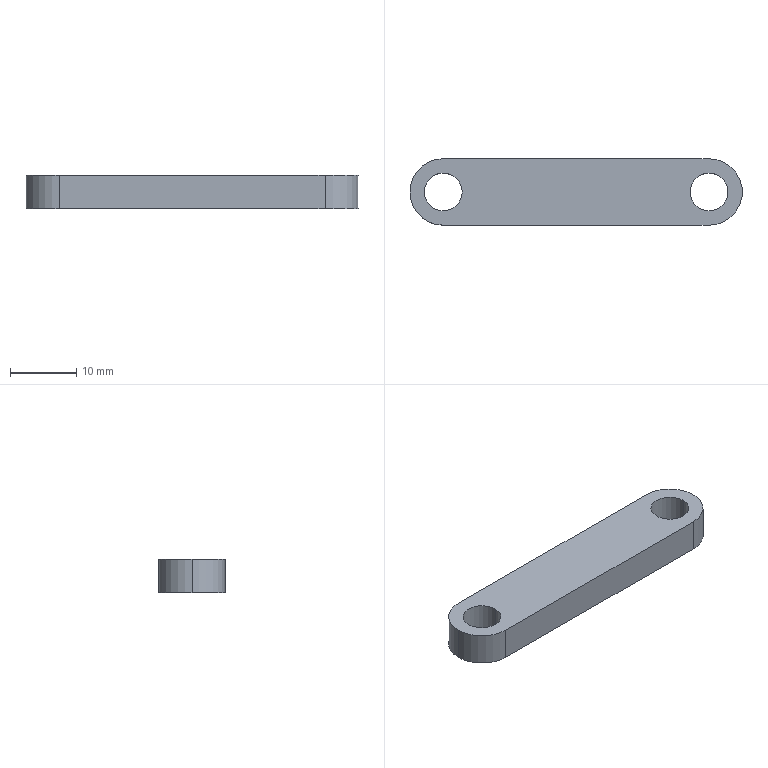Part | SolidWorks | features BaseBody 1 | 1 solid | 11 faces | box 50 x 10 x 5 mm | volume 2138 mm3 | cylinder 7 | plane 4 | commonest cylinder face diameters 5.7 x4 10 x3
STEP:
#1=CARTESIAN_POINT('',(17.15,0.,2.5));
#2=VERTEX_POINT('',#1);
#3=CARTESIAN_POINT('',(22.85,0.,2.5));
#4=VERTEX_POINT('',#3);
#5=CARTESIAN_POINT('',(20.,0.,2.5));
#6=DIRECTION('',(0.,0.,1.));
#7=DIRECTION('',(1.,0.,0.));
#8=AXIS2_PLACEMENT_3D('',#5,#6,#7);
#9=CIRCLE('',#8,2.85);
#10=EDGE_CURVE('',#2,#4,#9,.T.);
#11=ORIENTED_EDGE('',*,*,#10,.T.);
#12=CARTESIAN_POINT('',(22.85,0.,-2.5));
#13=VERTEX_POINT('',#12);
#14=CARTESIAN_POINT('',(22.85,0.,2.5));
#15=DIRECTION('',(0.,0.,-1.));
#16=VECTOR('',#15,1000.);
#17=LINE('',#14,#16);
#18=EDGE_CURVE('',#4,#13,#17,.T.);
#19=ORIENTED_EDGE('',*,*,#18,.T.);
#20=CARTESIAN_POINT('',(17.15,0.,-2.5));
#21=VERTEX_POINT('',#20);
#22=CARTESIAN_POINT('',(20.,0.,-2.5));
#23=DIRECTION('',(0.,0.,1.));
#24=DIRECTION('',(1.,0.,0.));
#25=AXIS2_PLACEMENT_3D('',#22,#23,#24);
#26=CIRCLE('',#25,2.85);
#27=EDGE_CURVE('',#21,#13,#26,.T.);
#28=ORIENTED_EDGE('',*,*,#27,.F.);
#29=CARTESIAN_POINT('',(17.15,0.,2.5));
#30=DIRECTION('',(0.,0.,-1.));
#31=VECTOR('',#30,1000.);
#32=LINE('',#29,#31);
#33=EDGE_CURVE('',#2,#21,#32,.T.);
#34=ORIENTED_EDGE('',*,*,#33,.F.);
#35=EDGE_LOOP('',(#11,#19,#28,#34));
#36=FACE_OUTER_BOUND('',#35,.T.);
#37=CARTESIAN_POINT('',(20.,0.,2.5));
#38=DIRECTION('',(0.,0.,-1.));
#39=DIRECTION('',(-1.,0.,0.));
#40=AXIS2_PLACEMENT_3D('',#37,#38,#39);
#41=CYLINDRICAL_SURFACE('',#40,2.85);
#42=ADVANCED_FACE('',(#36),#41,.F.);
#43=CARTESIAN_POINT('',(-22.85,0.,2.5));
#44=VERTEX_POINT('',#43);
#45=CARTESIAN_POINT('',(-17.15,0.,2.5));
#46=VERTEX_POINT('',#45);
#47=CARTESIAN_POINT('',(-20.,0.,2.5));
#48=DIRECTION('',(0.,0.,1.));
#49=DIRECTION('',(1.,0.,0.));
#50=AXIS2_PLACEMENT_3D('',#47,#48,#49);
#51=CIRCLE('',#50,2.85);
#52=EDGE_CURVE('',#44,#46,#51,.T.);
#53=ORIENTED_EDGE('',*,*,#52,.T.);
#54=CARTESIAN_POINT('',(-17.15,0.,-2.5));
#55=VERTEX_POINT('',#54);
#56=CARTESIAN_POINT('',(-17.15,0.,2.5));
#57=DIRECTION('',(0.,0.,-1.));
#58=VECTOR('',#57,1000.);
#59=LINE('',#56,#58);
#60=EDGE_CURVE('',#46,#55,#59,.T.);
#61=ORIENTED_EDGE('',*,*,#60,.T.);
#62=CARTESIAN_POINT('',(-22.85,0.,-2.5));
#63=VERTEX_POINT('',#62);
#64=CARTESIAN_POINT('',(-20.,0.,-2.5));
#65=DIRECTION('',(0.,0.,1.));
#66=DIRECTION('',(1.,0.,0.));
#67=AXIS2_PLACEMENT_3D('',#64,#65,#66);
#68=CIRCLE('',#67,2.85);
#69=EDGE_CURVE('',#63,#55,#68,.T.);
#70=ORIENTED_EDGE('',*,*,#69,.F.);
#71=CARTESIAN_POINT('',(-22.85,0.,2.5));
#72=DIRECTION('',(0.,0.,-1.));
#73=VECTOR('',#72,1000.);
#74=LINE('',#71,#73);
#75=EDGE_CURVE('',#44,#63,#74,.T.);
#76=ORIENTED_EDGE('',*,*,#75,.F.);
#77=EDGE_LOOP('',(#53,#61,#70,#76));
#78=FACE_OUTER_BOUND('',#77,.T.);
#79=CARTESIAN_POINT('',(-20.,0.,2.5));
#80=DIRECTION('',(0.,0.,-1.));
#81=DIRECTION('',(-1.,0.,0.));
#82=AXIS2_PLACEMENT_3D('',#79,#80,#81);
#83=CYLINDRICAL_SURFACE('',#82,2.85);
#84=ADVANCED_FACE('',(#78),#83,.F.);
#85=CARTESIAN_POINT('',(-25.,0.,2.5));
#86=VERTEX_POINT('',#85);
#87=CARTESIAN_POINT('',(-20.,-5.,2.5));
#88=VERTEX_POINT('',#87);
#89=CARTESIAN_POINT('',(-20.,0.,2.5));
#90=DIRECTION('',(0.,0.,1.));
#91=DIRECTION('',(1.,0.,0.));
#92=AXIS2_PLACEMENT_3D('',#89,#90,#91);
#93=CIRCLE('',#92,5.);
#94=EDGE_CURVE('',#86,#88,#93,.T.);
#95=ORIENTED_EDGE('',*,*,#94,.F.);
#96=CARTESIAN_POINT('',(-25.,0.,-2.5));
#97=VERTEX_POINT('',#96);
#98=CARTESIAN_POINT('',(-25.,0.,2.5));
#99=DIRECTION('',(0.,0.,-1.));
#100=VECTOR('',#99,1000.);
#101=LINE('',#98,#100);
#102=EDGE_CURVE('',#86,#97,#101,.T.);
#103=ORIENTED_EDGE('',*,*,#102,.T.);
#104=CARTESIAN_POINT('',(-20.,-5.,-2.5));
#105=VERTEX_POINT('',#104);
#106=CARTESIAN_POINT('',(-20.,0.,-2.5));
#107=DIRECTION('',(0.,0.,1.));
#108=DIRECTION('',(1.,0.,0.));
#109=AXIS2_PLACEMENT_3D('',#106,#107,#108);
#110=CIRCLE('',#109,5.);
#111=EDGE_CURVE('',#97,#105,#110,.T.);
#112=ORIENTED_EDGE('',*,*,#111,.T.);
#113=CARTESIAN_POINT('',(-20.,-5.,2.5));
#114=DIRECTION('',(0.,0.,-1.));
#115=VECTOR('',#114,1000.);
#116=LINE('',#113,#115);
#117=EDGE_CURVE('',#88,#105,#116,.T.);
#118=ORIENTED_EDGE('',*,*,#117,.F.);
#119=EDGE_LOOP('',(#95,#103,#112,#118));
#120=FACE_OUTER_BOUND('',#119,.T.);
#121=CARTESIAN_POINT('',(-20.,0.,2.5));
#122=DIRECTION('',(0.,0.,-1.));
#123=DIRECTION('',(-1.,0.,0.));
#124=AXIS2_PLACEMENT_3D('',#121,#122,#123);
#125=CYLINDRICAL_SURFACE('',#124,5.);
#126=ADVANCED_FACE('',(#120),#125,.T.);
#127=ORIENTED_EDGE('',*,*,#52,.F.);
#128=CARTESIAN_POINT('',(-20.,0.,2.5));
#129=DIRECTION('',(0.,0.,1.));
#130=DIRECTION('',(1.,0.,0.));
#131=AXIS2_PLACEMENT_3D('',#128,#129,#130);
#132=CIRCLE('',#131,2.85);
#133=EDGE_CURVE('',#46,#44,#132,.T.);
#134=ORIENTED_EDGE('',*,*,#133,.F.);
#135=EDGE_LOOP('',(#127,#134));
#136=FACE_BOUND('',#135,.T.);
#137=CARTESIAN_POINT('',(-20.,5.,2.5));
#138=VERTEX_POINT('',#137);
#139=CARTESIAN_POINT('',(-20.,0.,2.5));
#140=DIRECTION('',(0.,0.,1.));
#141=DIRECTION('',(1.,0.,0.));
#142=AXIS2_PLACEMENT_3D('',#139,#140,#141);
#143=CIRCLE('',#142,5.);
#144=EDGE_CURVE('',#138,#86,#143,.T.);
#145=ORIENTED_EDGE('',*,*,#144,.T.);
#146=ORIENTED_EDGE('',*,*,#94,.T.);
#147=CARTESIAN_POINT('',(20.,-5.,2.5));
#148=VERTEX_POINT('',#147);
#149=CARTESIAN_POINT('',(-20.,-5.,2.5));
#150=DIRECTION('',(1.,0.,0.));
#151=VECTOR('',#150,1000.);
#152=LINE('',#149,#151);
#153=EDGE_CURVE('',#88,#148,#152,.T.);
#154=ORIENTED_EDGE('',*,*,#153,.T.);
#155=CARTESIAN_POINT('',(20.,5.,2.5));
#156=VERTEX_POINT('',#155);
#157=CARTESIAN_POINT('',(20.,0.,2.5));
#158=DIRECTION('',(0.,0.,1.));
#159=DIRECTION('',(1.,0.,0.));
#160=AXIS2_PLACEMENT_3D('',#157,#158,#159);
#161=CIRCLE('',#160,5.);
#162=EDGE_CURVE('',#148,#156,#161,.T.);
#163=ORIENTED_EDGE('',*,*,#162,.T.);
#164=CARTESIAN_POINT('',(-20.,5.,2.5));
#165=DIRECTION('',(-1.,0.,0.));
#166=VECTOR('',#165,1000.);
#167=LINE('',#164,#166);
#168=EDGE_CURVE('',#156,#138,#167,.T.);
#169=ORIENTED_EDGE('',*,*,#168,.T.);
#170=EDGE_LOOP('',(#145,#146,#154,#163,#169));
#171=FACE_OUTER_BOUND('',#170,.T.);
#172=ORIENTED_EDGE('',*,*,#10,.F.);
#173=CARTESIAN_POINT('',(20.,0.,2.5));
#174=DIRECTION('',(0.,0.,1.));
#175=DIRECTION('',(1.,0.,0.));
#176=AXIS2_PLACEMENT_3D('',#173,#174,#175);
#177=CIRCLE('',#176,2.85);
#178=EDGE_CURVE('',#4,#2,#177,.T.);
#179=ORIENTED_EDGE('',*,*,#178,.F.);
#180=EDGE_LOOP('',(#172,#179));
#181=FACE_BOUND('',#180,.T.);
#182=CARTESIAN_POINT('',(-20.,0.,2.5));
#183=DIRECTION('',(0.,0.,1.));
#184=DIRECTION('',(1.,0.,0.));
#185=AXIS2_PLACEMENT_3D('',#182,#183,#184);
#186=PLANE('',#185);
#187=ADVANCED_FACE('',(#136,#171,#181),#186,.T.);
#188=CARTESIAN_POINT('',(-20.,5.,-2.5));
#189=VERTEX_POINT('',#188);
#190=CARTESIAN_POINT('',(-20.,0.,-2.5));
#191=DIRECTION('',(0.,0.,1.));
#192=DIRECTION('',(1.,0.,0.));
#193=AXIS2_PLACEMENT_3D('',#190,#191,#192);
#194=CIRCLE('',#193,5.);
#195=EDGE_CURVE('',#189,#97,#194,.T.);
#196=ORIENTED_EDGE('',*,*,#195,.F.);
#197=CARTESIAN_POINT('',(20.,5.,-2.5));
#198=VERTEX_POINT('',#197);
#199=CARTESIAN_POINT('',(-20.,5.,-2.5));
#200=DIRECTION('',(-1.,0.,0.));
#201=VECTOR('',#200,1000.);
#202=LINE('',#199,#201);
#203=EDGE_CURVE('',#198,#189,#202,.T.);
#204=ORIENTED_EDGE('',*,*,#203,.F.);
#205=CARTESIAN_POINT('',(20.,-5.,-2.5));
#206=VERTEX_POINT('',#205);
#207=CARTESIAN_POINT('',(20.,0.,-2.5));
#208=DIRECTION('',(0.,0.,1.));
#209=DIRECTION('',(1.,0.,0.));
#210=AXIS2_PLACEMENT_3D('',#207,#208,#209);
#211=CIRCLE('',#210,5.);
#212=EDGE_CURVE('',#206,#198,#211,.T.);
#213=ORIENTED_EDGE('',*,*,#212,.F.);
#214=CARTESIAN_POINT('',(-20.,-5.,-2.5));
#215=DIRECTION('',(1.,0.,0.));
#216=VECTOR('',#215,1000.);
#217=LINE('',#214,#216);
#218=EDGE_CURVE('',#105,#206,#217,.T.);
#219=ORIENTED_EDGE('',*,*,#218,.F.);
#220=ORIENTED_EDGE('',*,*,#111,.F.);
#221=EDGE_LOOP('',(#196,#204,#213,#219,#220));
#222=FACE_OUTER_BOUND('',#221,.T.);
#223=ORIENTED_EDGE('',*,*,#69,.T.);
#224=CARTESIAN_POINT('',(-20.,0.,-2.5));
#225=DIRECTION('',(0.,0.,1.));
#226=DIRECTION('',(1.,0.,0.));
#227=AXIS2_PLACEMENT_3D('',#224,#225,#226);
#228=CIRCLE('',#227,2.85);
#229=EDGE_CURVE('',#55,#63,#228,.T.);
#230=ORIENTED_EDGE('',*,*,#229,.T.);
#231=EDGE_LOOP('',(#223,#230));
#232=FACE_BOUND('',#231,.T.);
#233=ORIENTED_EDGE('',*,*,#27,.T.);
#234=CARTESIAN_POINT('',(20.,0.,-2.5));
#235=DIRECTION('',(0.,0.,1.));
#236=DIRECTION('',(1.,0.,0.));
#237=AXIS2_PLACEMENT_3D('',#234,#235,#236);
#238=CIRCLE('',#237,2.85);
#239=EDGE_CURVE('',#13,#21,#238,.T.);
#240=ORIENTED_EDGE('',*,*,#239,.T.);
#241=EDGE_LOOP('',(#233,#240));
#242=FACE_BOUND('',#241,.T.);
#243=CARTESIAN_POINT('',(-20.,0.,-2.5));
#244=DIRECTION('',(0.,0.,1.));
#245=DIRECTION('',(1.,0.,0.));
#246=AXIS2_PLACEMENT_3D('',#243,#244,#245);
#247=PLANE('',#246);
#248=ADVANCED_FACE('',(#222,#232,#242),#247,.F.);
#249=ORIENTED_EDGE('',*,*,#102,.F.);
#250=ORIENTED_EDGE('',*,*,#144,.F.);
#251=CARTESIAN_POINT('',(-20.,5.,2.5));
#252=DIRECTION('',(0.,0.,-1.));
#253=VECTOR('',#252,1000.);
#254=LINE('',#251,#253);
#255=EDGE_CURVE('',#138,#189,#254,.T.);
#256=ORIENTED_EDGE('',*,*,#255,.T.);
#257=ORIENTED_EDGE('',*,*,#195,.T.);
#258=EDGE_LOOP('',(#249,#250,#256,#257));
#259=FACE_OUTER_BOUND('',#258,.T.);
#260=CARTESIAN_POINT('',(-20.,0.,2.5));
#261=DIRECTION('',(0.,0.,-1.));
#262=DIRECTION('',(-1.,0.,0.));
#263=AXIS2_PLACEMENT_3D('',#260,#261,#262);
#264=CYLINDRICAL_SURFACE('',#263,5.);
#265=ADVANCED_FACE('',(#259),#264,.T.);
#266=ORIENTED_EDGE('',*,*,#218,.T.);
#267=CARTESIAN_POINT('',(20.,-5.,2.5));
#268=DIRECTION('',(0.,0.,-1.));
#269=VECTOR('',#268,1000.);
#270=LINE('',#267,#269);
#271=EDGE_CURVE('',#148,#206,#270,.T.);
#272=ORIENTED_EDGE('',*,*,#271,.F.);
#273=ORIENTED_EDGE('',*,*,#153,.F.);
#274=ORIENTED_EDGE('',*,*,#117,.T.);
#275=EDGE_LOOP('',(#266,#272,#273,#274));
#276=FACE_OUTER_BOUND('',#275,.T.);
#277=CARTESIAN_POINT('',(-20.,-5.,2.5));
#278=DIRECTION('',(0.,1.,0.));
#279=DIRECTION('',(-1.,0.,0.));
#280=AXIS2_PLACEMENT_3D('',#277,#278,#279);
#281=PLANE('',#280);
#282=ADVANCED_FACE('',(#276),#281,.F.);
#283=ORIENTED_EDGE('',*,*,#212,.T.);
#284=CARTESIAN_POINT('',(20.,5.,2.5));
#285=DIRECTION('',(0.,0.,-1.));
#286=VECTOR('',#285,1000.);
#287=LINE('',#284,#286);
#288=EDGE_CURVE('',#156,#198,#287,.T.);
#289=ORIENTED_EDGE('',*,*,#288,.F.);
#290=ORIENTED_EDGE('',*,*,#162,.F.);
#291=ORIENTED_EDGE('',*,*,#271,.T.);
#292=EDGE_LOOP('',(#283,#289,#290,#291));
#293=FACE_OUTER_BOUND('',#292,.T.);
#294=CARTESIAN_POINT('',(20.,0.,2.5));
#295=DIRECTION('',(0.,0.,-1.));
#296=DIRECTION('',(-1.,0.,0.));
#297=AXIS2_PLACEMENT_3D('',#294,#295,#296);
#298=CYLINDRICAL_SURFACE('',#297,5.);
#299=ADVANCED_FACE('',(#293),#298,.T.);
#300=ORIENTED_EDGE('',*,*,#203,.T.);
#301=ORIENTED_EDGE('',*,*,#255,.F.);
#302=ORIENTED_EDGE('',*,*,#168,.F.);
#303=ORIENTED_EDGE('',*,*,#288,.T.);
#304=EDGE_LOOP('',(#300,#301,#302,#303));
#305=FACE_OUTER_BOUND('',#304,.T.);
#306=CARTESIAN_POINT('',(-20.,5.,2.5));
#307=DIRECTION('',(0.,-1.,0.));
#308=DIRECTION('',(1.,0.,0.));
#309=AXIS2_PLACEMENT_3D('',#306,#307,#308);
#310=PLANE('',#309);
#311=ADVANCED_FACE('',(#305),#310,.F.);
#312=ORIENTED_EDGE('',*,*,#60,.F.);
#313=ORIENTED_EDGE('',*,*,#133,.T.);
#314=ORIENTED_EDGE('',*,*,#75,.T.);
#315=ORIENTED_EDGE('',*,*,#229,.F.);
#316=EDGE_LOOP('',(#312,#313,#314,#315));
#317=FACE_OUTER_BOUND('',#316,.T.);
#318=CARTESIAN_POINT('',(-20.,0.,2.5));
#319=DIRECTION('',(0.,0.,-1.));
#320=DIRECTION('',(-1.,0.,0.));
#321=AXIS2_PLACEMENT_3D('',#318,#319,#320);
#322=CYLINDRICAL_SURFACE('',#321,2.85);
#323=ADVANCED_FACE('',(#317),#322,.F.);
#324=ORIENTED_EDGE('',*,*,#18,.F.);
#325=ORIENTED_EDGE('',*,*,#178,.T.);
#326=ORIENTED_EDGE('',*,*,#33,.T.);
#327=ORIENTED_EDGE('',*,*,#239,.F.);
#328=EDGE_LOOP('',(#324,#325,#326,#327));
#329=FACE_OUTER_BOUND('',#328,.T.);
#330=CARTESIAN_POINT('',(20.,0.,2.5));
#331=DIRECTION('',(0.,0.,-1.));
#332=DIRECTION('',(-1.,0.,0.));
#333=AXIS2_PLACEMENT_3D('',#330,#331,#332);
#334=CYLINDRICAL_SURFACE('',#333,2.85);
#335=ADVANCED_FACE('',(#329),#334,.F.);
#336=CLOSED_SHELL('',(#42,#84,#126,#187,#248,#265,#282,#299,#311,#323,#335));
#337=MANIFOLD_SOLID_BREP('',#336);
#338=CARTESIAN_POINT('',(0.,0.,0.));
#339=DIRECTION('',(0.,0.,1.));
#340=DIRECTION('',(1.,0.,0.));
#341=AXIS2_PLACEMENT_3D('',#338,#339,#340);
#342=(LENGTH_UNIT()NAMED_UNIT(*)SI_UNIT(.MILLI.,.METRE.));
#343=UNCERTAINTY_MEASURE_WITH_UNIT(LENGTH_MEASURE(0.00001),#342,'','');
#344=(NAMED_UNIT(*)PLANE_ANGLE_UNIT()SI_UNIT($,.RADIAN.));
#345=(NAMED_UNIT(*)SI_UNIT($,.STERADIAN.)SOLID_ANGLE_UNIT());
#346=(GEOMETRIC_REPRESENTATION_CONTEXT(3)GLOBAL_UNCERTAINTY_ASSIGNED_CONTEXT((#343))GLOBAL_UNIT_ASSIGNED_CONTEXT((#342,#344,#345))REPRESENTATION_CONTEXT('',''));
#347=ADVANCED_BREP_SHAPE_REPRESENTATION('',(#337,#341),#346);